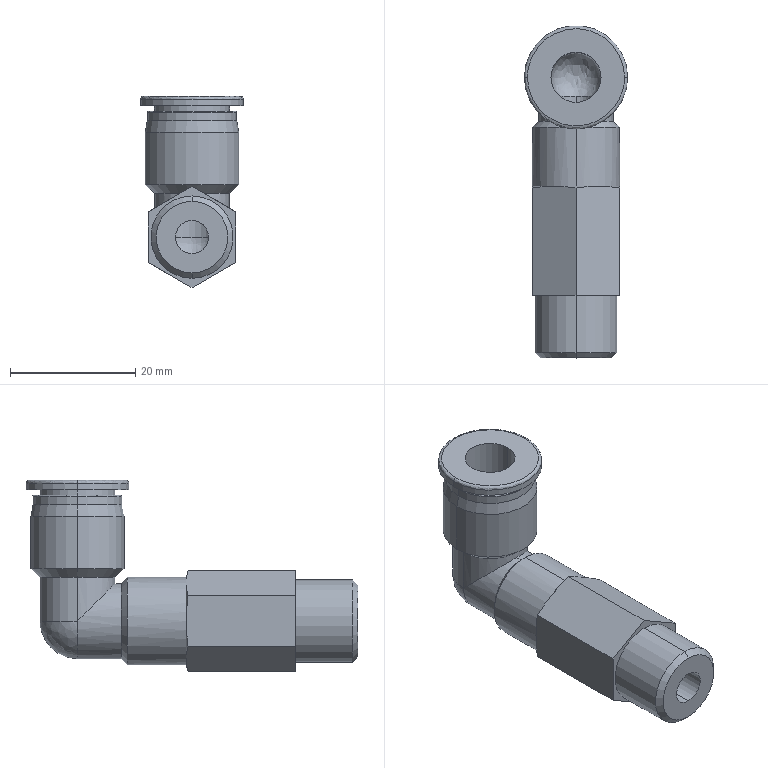Part | STEP file | APLL08-02 | 1 solid | 52 faces | box 16.5 x 53.05 x 30.583 mm | volume 7861 mm3 | cylinder 20 | cone 15 | plane 11 | spline 6 | commonest cylinder face diameters 12 x6 5.333 x2 8 x2 13.157 x2 14 x2 14.25 x2